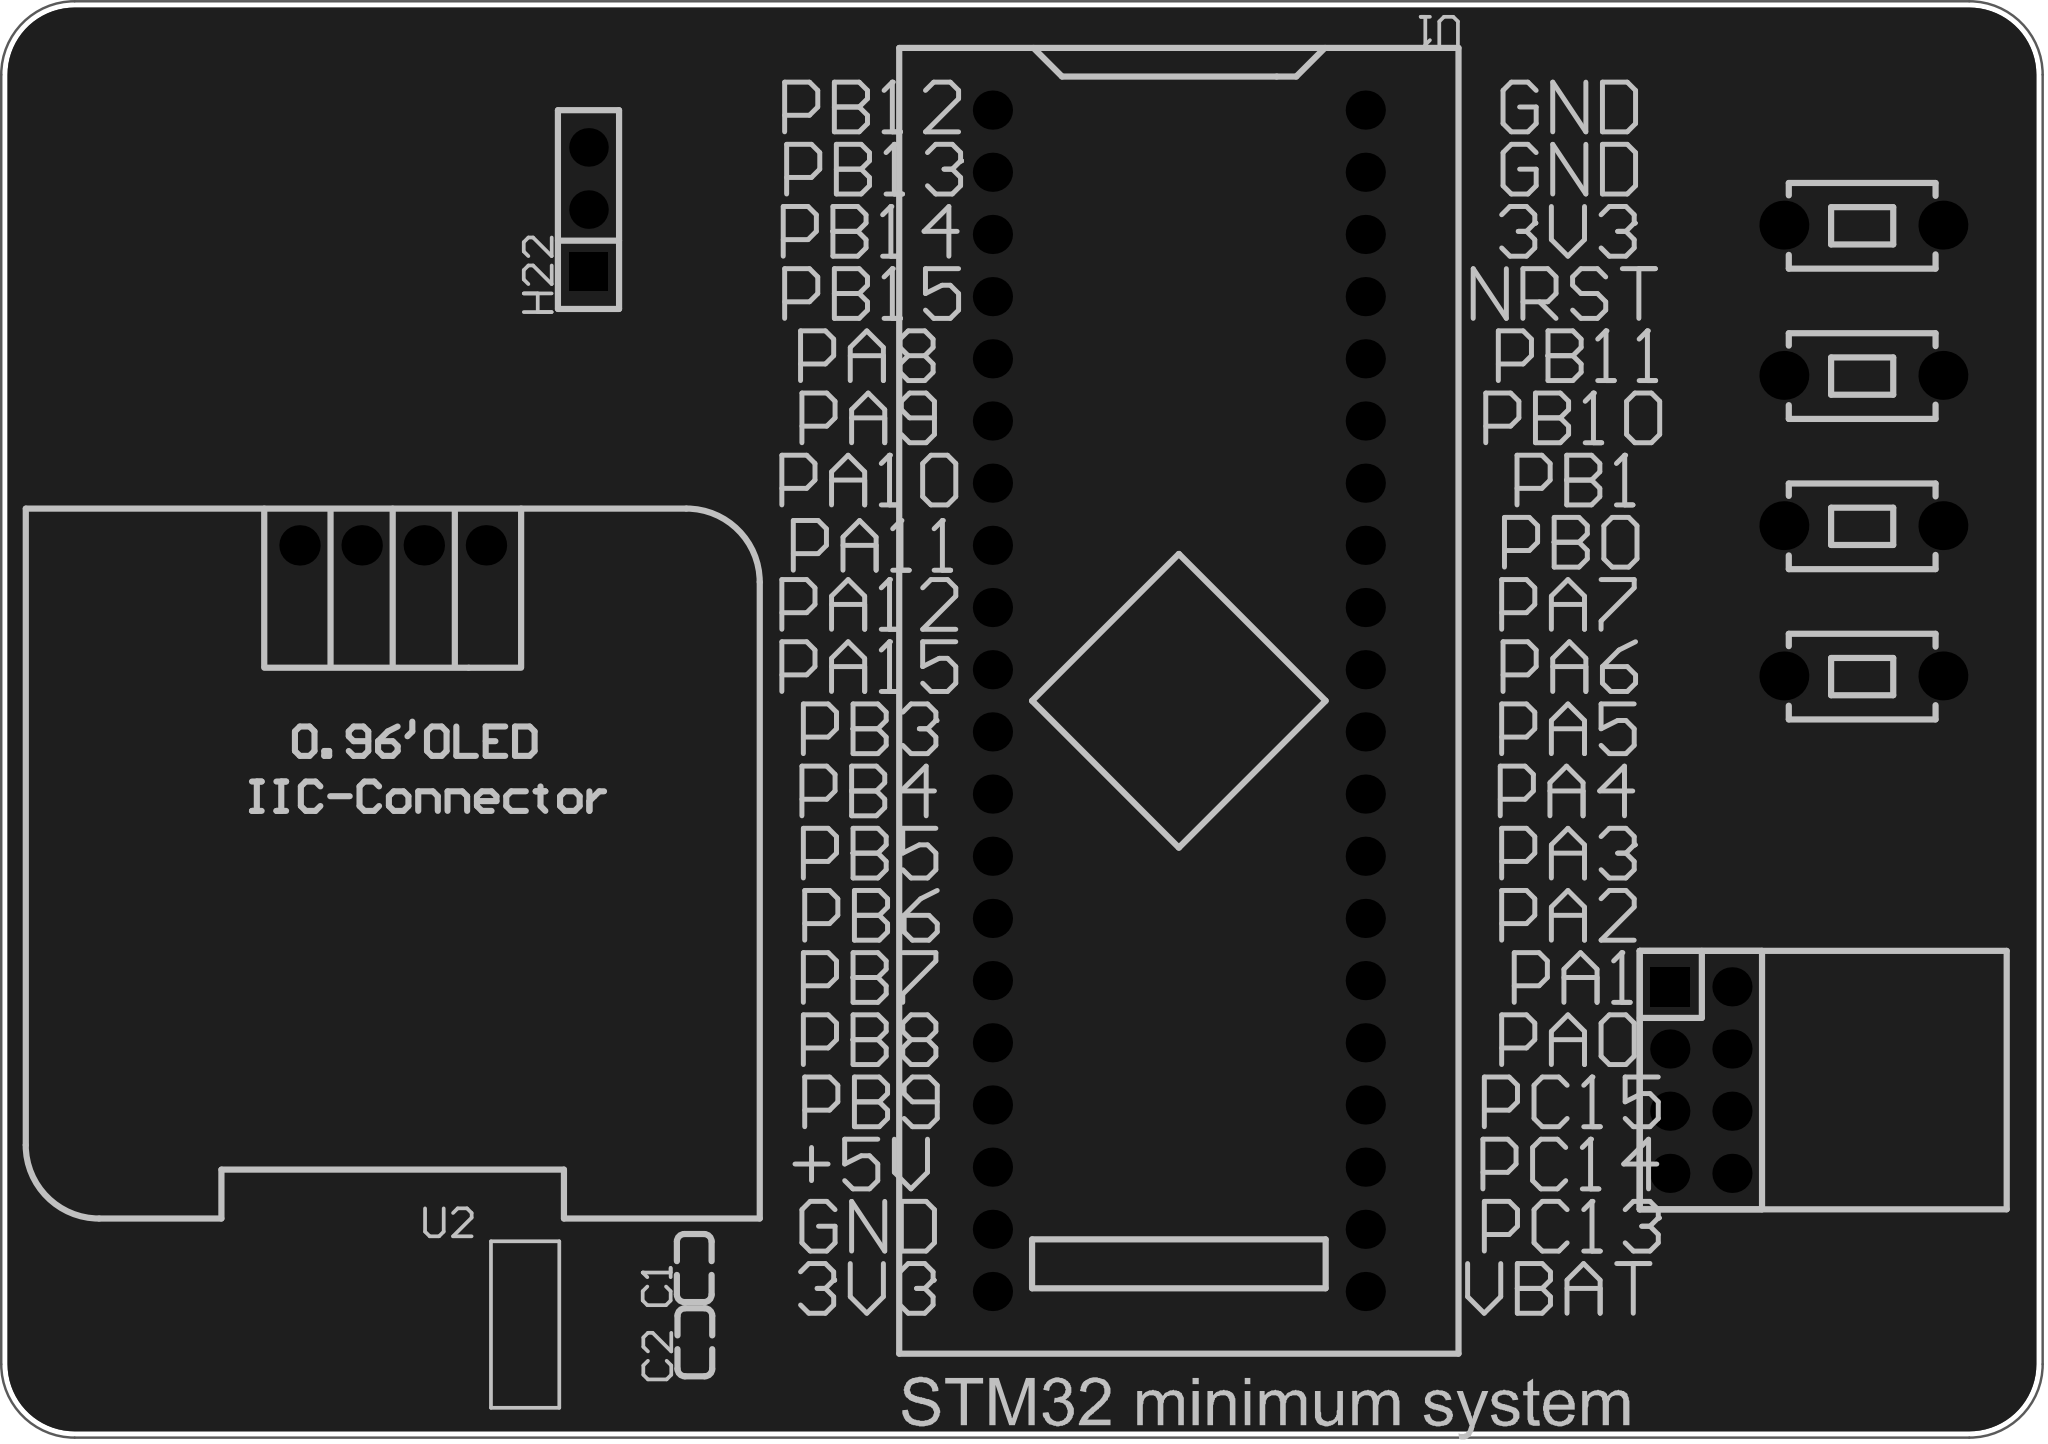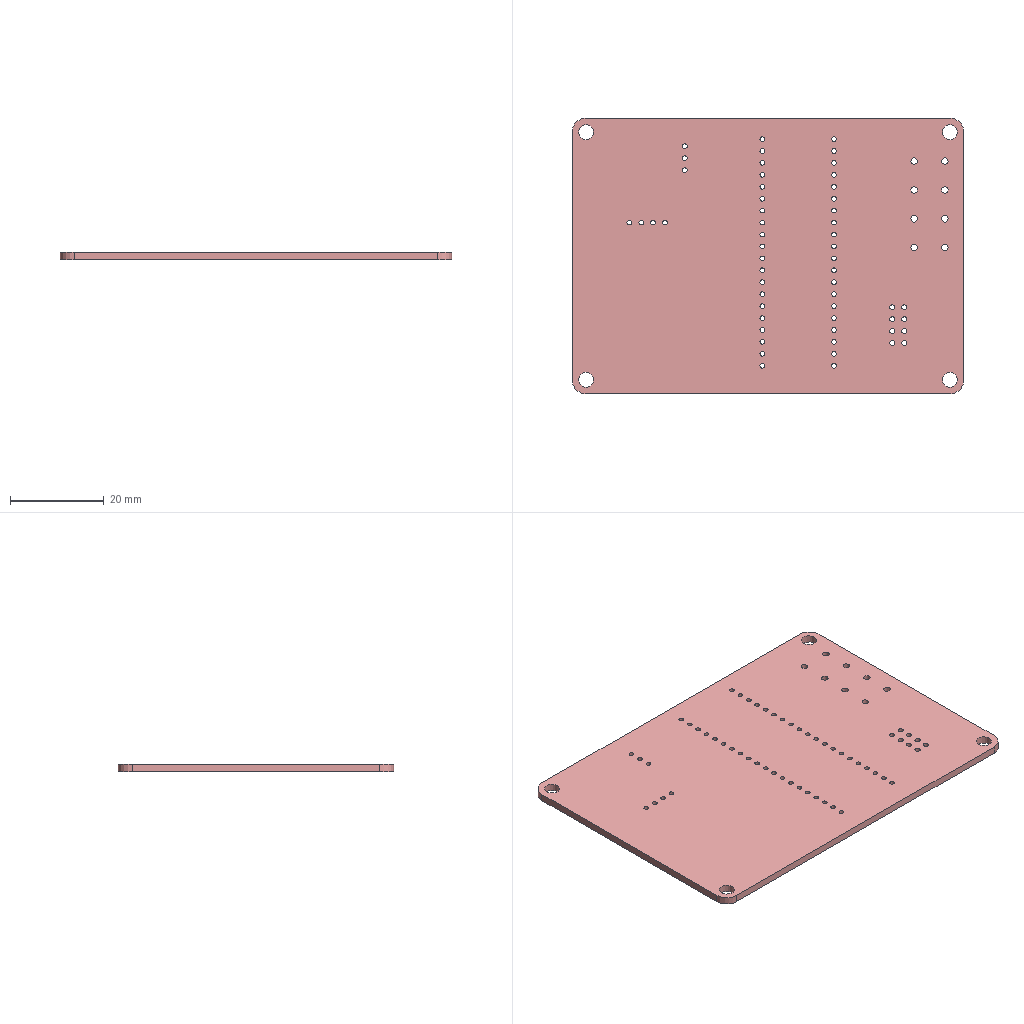Circuit board layout | Altium Designer | box 83.4 x 58.7 x 1.6 mm
Layer stack:
# Altium Designer layer stack of  (unit mm; dielectric type: 0 none, 1 core, 2 prepreg, 3 surface material)
index,name,kind,layer,copper_thickness_mm,dielectric_type,dielectric_thickness_mm,dielectric_material,dielectric_constant
0,Top Paste Mask Layer,other,,,,,,
1,Top Silkscreen Layer,other,,,,,,
2,Top Solder Mask Layer,dielectric,,,3,0.01,,3.3
3,Top Layer,copper,Top Layer,0.035,,,,
4,Dielectric1,dielectric,,,3,1.51,FR4,4.5
5,Bottom Layer,copper,Bottom Layer,0.035,,,,
6,Bottom Solder Mask Layer,dielectric,,,3,0.01,,3.3
7,Bottom Silkscreen Layer,other,,,,,,
8,Bottom Paste Mask Layer,other,,,,,,
# drill layer pairs: low layer,high layer
drill_pair,Top Layer,Bottom Layer
Part placement:
Designator,Comment,Layer,Footprint,Center-X(mm),Center-Y(mm),Rotation
U1,STM32F103C8T6-Card,TopLayer,CONN-TH_L53.3-W22.9_STM32F103C8T6-CARD,132.715,135.382,270
C1,100nF,TopLayer,C0603,112.907,112.21,90
C2,100nF,TopLayer,C0603,112.933,109.177,90
OLED1,,TopLayer,0.96OLED_4P,100.584,141.732,0
H22,,TopLayer,HDR-TH_3P-P2.54-V-F,108.585,155.448,90
SW8,,TopLayer,Key_TH_3.5x6x4.3,160.693,136.398,0
H16,,TopLayer,HDR-TH_8P-P2.54-V-F-R2-C4-S2.54-1,154.051,119.888,270
SW9,,TopLayer,Key_TH_3.5x6x4.3,160.693,142.536,0
SW10,,TopLayer,Key_TH_3.5x6x4.3,160.693,148.675,0
SW11,,TopLayer,Key_TH_3.5x6x4.3,160.693,154.813,0
U2,AMS1117-5.0,TopLayer,SOT-223_L6.5-W3.5-P2.30-LS7.0-BR,105.995,109.903,0
Pad and via stacks:
# Altium Designer via and pad stacks of  (unit mm). Each distinct definition once, with the count of objects using it.
# via: kind,start_layer,end_layer,hole_mm,diameter_mm,mode(0 simple;1 top-mid-bottom;2 full stack),diameter_per_layer,count,example_net
# pad: kind,layer,hole_mm,hole_type(0 round;1 square;2 slot),plating,top_size,top_shape(1 round;2 rect;3 octagon;9 rounded rect),mid_size,bottom_size,mode,footprint,size_per_layer,count,example
pad,Multi-Layer,1,0,plated,1.6x1.6,1,1.6x1.6,1.6x1.6,0,CONN-TH_L53.3-W22.9_STM32F103C8T6-CARD,,40,U1.1
pad,Multi-Layer,1,0,plated,1.65x1.65,1,1.65x1.65,1.65x1.65,0,0.96OLED_4P,,4,OLED1.4
pad,Multi-Layer,1.02,0,plated,1.575x1.575,1,1.575x1.575,1.575x1.575,0,HDR-TH_3P-P2.54-V-F,,2,H22.3
pad,Multi-Layer,1.02,0,plated,1.575x1.575,2,1.575x1.575,1.575x1.575,0,HDR-TH_3P-P2.54-V-F,,1,H22.1
pad,Multi-Layer,1.399,0,plated,1.999x1.999,1,1.999x1.999,1.999x1.999,0,Key_TH_3.5x6x4.3,,8,SW8.A
pad,Multi-Layer,1.1,0,plated,1.6x1.6,2,1.6x1.6,1.6x1.6,0,HDR-TH_8P-P2.54-V-F-R2-C4-S2.54-1,,1,H16.1
pad,Multi-Layer,1.1,0,plated,1.6x1.6,1,1.6x1.6,1.6x1.6,0,HDR-TH_8P-P2.54-V-F-R2-C4-S2.54-1,,7,H16.2
pad,Top Layer,0,0,plated,0.8x0.9,2,0.8x0.9,0.8x0.9,0,C0603,,4,C1.2
pad,Top Layer,0,0,plated,2.465x1.05,2,2.465x1.05,2.465x1.05,0,SOT-223_L6.5-W3.5-P2.30-LS7.0-BR,,3,U2.1
pad,Top Layer,0,0,plated,2.465x3.54,2,2.465x3.54,2.465x3.54,0,SOT-223_L6.5-W3.5-P2.30-LS7.0-BR,,1,U2.4
Copper pours:
name,layer,net,type(0 solid;1 hatched;2 none)
Bottom Layer-GND,Bottom Layer,GND,0
Top Layer-GND,Top Layer,GND,0
Design rules, without the lines most boards share:
# Altium Designer design rules of  (exported by Altium Designer, unit mm)
# columns: name | kind | enabled | priority | scope1 | scope2 | descriptor | typed fields (field=value)
copperThickness1oz_2 | 2 | enabled | 2 | All | All | Width Constraint (Min=5mil) (Max=100mil) (Preferred=30mil) (All) |
viaSize | 11 | enabled | 1 | All | All | Routing Via (MinHoleWidth=11.811mil) (MaxHoleWidth=248.032mil) (PreferredHoleWidth=12.008mil) (MinWidth=19.685mil) (MaxWidth=393.701mil) (PreferedWidth=24.016mil) (All) | via_min_hole=0.3 via_max_hole=6.3 via_preferred_diameter=0.61 via_preferred_hole=0.305
solderMaskExpansion | 13 | enabled | 2 | All | All | Solder Mask Expansion (Expansion =2.008mil) (All) | expansion=0.051